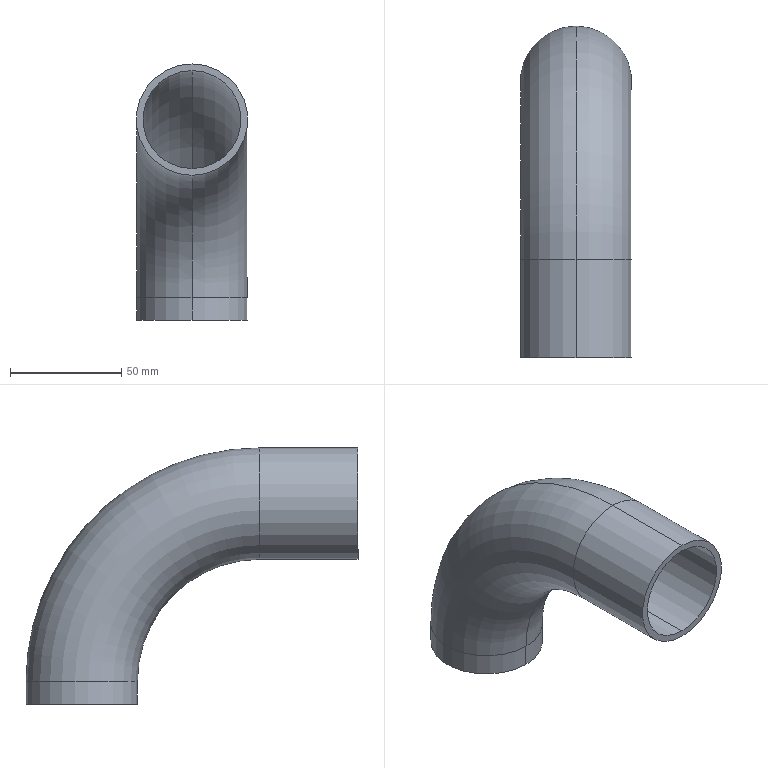Part | SolidWorks | features BaseBody 1 | 1 solid | 14 faces | box 50 x 149 x 115 mm | volume 79585 mm3 | cylinder 8 | torus 4 | plane 2 | commonest cylinder face diameters 44 x4 50 x4
STEP:
#1=CARTESIAN_POINT('',(0.,75.,-80.));
#2=VERTEX_POINT('',#1);
#3=CARTESIAN_POINT('',(0.,125.,-80.));
#4=VERTEX_POINT('',#3);
#5=CARTESIAN_POINT('',(0.,100.,-80.));
#6=DIRECTION('',(0.,0.,1.));
#7=DIRECTION('',(0.,-1.,0.));
#8=AXIS2_PLACEMENT_3D('',#5,#6,#7);
#9=CIRCLE('',#8,25.);
#10=EDGE_CURVE('',#2,#4,#9,.T.);
#11=ORIENTED_EDGE('',*,*,#10,.T.);
#12=CARTESIAN_POINT('',(0.,20.,25.));
#13=VERTEX_POINT('',#12);
#14=CARTESIAN_POINT('',(0.,20.,-80.));
#15=DIRECTION('',(1.,0.,0.));
#16=DIRECTION('',(0.,0.,-1.));
#17=AXIS2_PLACEMENT_3D('',#14,#15,#16);
#18=CIRCLE('',#17,105.);
#19=EDGE_CURVE('',#4,#13,#18,.T.);
#20=ORIENTED_EDGE('',*,*,#19,.T.);
#21=CARTESIAN_POINT('',(0.,20.,-25.));
#22=VERTEX_POINT('',#21);
#23=CARTESIAN_POINT('',(0.,20.,0.));
#24=DIRECTION('',(0.,-1.,0.));
#25=DIRECTION('',(0.,0.,-1.));
#26=AXIS2_PLACEMENT_3D('',#23,#24,#25);
#27=CIRCLE('',#26,25.);
#28=EDGE_CURVE('',#22,#13,#27,.T.);
#29=ORIENTED_EDGE('',*,*,#28,.F.);
#30=CARTESIAN_POINT('',(0.,20.,-80.));
#31=DIRECTION('',(1.,0.,0.));
#32=DIRECTION('',(0.,0.,-1.));
#33=AXIS2_PLACEMENT_3D('',#30,#31,#32);
#34=CIRCLE('',#33,55.);
#35=EDGE_CURVE('',#2,#22,#34,.T.);
#36=ORIENTED_EDGE('',*,*,#35,.F.);
#37=EDGE_LOOP('',(#11,#20,#29,#36));
#38=FACE_OUTER_BOUND('',#37,.T.);
#39=CARTESIAN_POINT('',(0.,20.,-80.));
#40=DIRECTION('',(1.,0.,0.));
#41=DIRECTION('',(0.,0.,1.));
#42=AXIS2_PLACEMENT_3D('',#39,#40,#41);
#43=TOROIDAL_SURFACE('',#42,80.,25.);
#44=ADVANCED_FACE('',(#38),#43,.T.);
#45=CARTESIAN_POINT('',(0.,122.,-80.));
#46=VERTEX_POINT('',#45);
#47=CARTESIAN_POINT('',(0.,78.,-80.));
#48=VERTEX_POINT('',#47);
#49=CARTESIAN_POINT('',(0.,100.,-80.));
#50=DIRECTION('',(0.,0.,1.));
#51=DIRECTION('',(0.,-1.,0.));
#52=AXIS2_PLACEMENT_3D('',#49,#50,#51);
#53=CIRCLE('',#52,22.);
#54=EDGE_CURVE('',#46,#48,#53,.T.);
#55=ORIENTED_EDGE('',*,*,#54,.F.);
#56=CARTESIAN_POINT('',(0.,20.,22.));
#57=VERTEX_POINT('',#56);
#58=CARTESIAN_POINT('',(0.,20.,-80.));
#59=DIRECTION('',(1.,0.,0.));
#60=DIRECTION('',(0.,0.,-1.));
#61=AXIS2_PLACEMENT_3D('',#58,#59,#60);
#62=CIRCLE('',#61,102.);
#63=EDGE_CURVE('',#46,#57,#62,.T.);
#64=ORIENTED_EDGE('',*,*,#63,.T.);
#65=CARTESIAN_POINT('',(0.,20.,-22.));
#66=VERTEX_POINT('',#65);
#67=CARTESIAN_POINT('',(0.,20.,0.));
#68=DIRECTION('',(0.,-1.,0.));
#69=DIRECTION('',(0.,0.,-1.));
#70=AXIS2_PLACEMENT_3D('',#67,#68,#69);
#71=CIRCLE('',#70,22.);
#72=EDGE_CURVE('',#57,#66,#71,.T.);
#73=ORIENTED_EDGE('',*,*,#72,.T.);
#74=CARTESIAN_POINT('',(0.,20.,-80.));
#75=DIRECTION('',(1.,0.,0.));
#76=DIRECTION('',(0.,0.,-1.));
#77=AXIS2_PLACEMENT_3D('',#74,#75,#76);
#78=CIRCLE('',#77,58.);
#79=EDGE_CURVE('',#48,#66,#78,.T.);
#80=ORIENTED_EDGE('',*,*,#79,.F.);
#81=EDGE_LOOP('',(#55,#64,#73,#80));
#82=FACE_OUTER_BOUND('',#81,.T.);
#83=CARTESIAN_POINT('',(0.,20.,-80.));
#84=DIRECTION('',(1.,0.,0.));
#85=DIRECTION('',(0.,0.,1.));
#86=AXIS2_PLACEMENT_3D('',#83,#84,#85);
#87=TOROIDAL_SURFACE('',#86,80.,22.);
#88=ADVANCED_FACE('',(#82),#87,.F.);
#89=CARTESIAN_POINT('',(0.,20.,0.));
#90=DIRECTION('',(0.,-1.,0.));
#91=DIRECTION('',(0.,0.,-1.));
#92=AXIS2_PLACEMENT_3D('',#89,#90,#91);
#93=CIRCLE('',#92,25.);
#94=EDGE_CURVE('',#13,#22,#93,.T.);
#95=ORIENTED_EDGE('',*,*,#94,.T.);
#96=CARTESIAN_POINT('',(0.,-24.,-25.));
#97=VERTEX_POINT('',#96);
#98=CARTESIAN_POINT('',(0.,20.,-25.));
#99=DIRECTION('',(0.,-1.,0.));
#100=VECTOR('',#99,1000.);
#101=LINE('',#98,#100);
#102=EDGE_CURVE('',#22,#97,#101,.T.);
#103=ORIENTED_EDGE('',*,*,#102,.T.);
#104=CARTESIAN_POINT('',(0.,-24.,25.));
#105=VERTEX_POINT('',#104);
#106=CARTESIAN_POINT('',(0.,-24.,0.));
#107=DIRECTION('',(0.,-1.,0.));
#108=DIRECTION('',(0.,0.,-1.));
#109=AXIS2_PLACEMENT_3D('',#106,#107,#108);
#110=CIRCLE('',#109,25.);
#111=EDGE_CURVE('',#105,#97,#110,.T.);
#112=ORIENTED_EDGE('',*,*,#111,.F.);
#113=CARTESIAN_POINT('',(0.,20.,25.));
#114=DIRECTION('',(0.,-1.,0.));
#115=VECTOR('',#114,1000.);
#116=LINE('',#113,#115);
#117=EDGE_CURVE('',#13,#105,#116,.T.);
#118=ORIENTED_EDGE('',*,*,#117,.F.);
#119=EDGE_LOOP('',(#95,#103,#112,#118));
#120=FACE_OUTER_BOUND('',#119,.T.);
#121=CARTESIAN_POINT('',(0.,20.,0.));
#122=DIRECTION('',(0.,-1.,0.));
#123=DIRECTION('',(0.,0.,1.));
#124=AXIS2_PLACEMENT_3D('',#121,#122,#123);
#125=CYLINDRICAL_SURFACE('',#124,25.);
#126=ADVANCED_FACE('',(#120),#125,.T.);
#127=CARTESIAN_POINT('',(0.,20.,0.));
#128=DIRECTION('',(0.,-1.,0.));
#129=DIRECTION('',(0.,0.,-1.));
#130=AXIS2_PLACEMENT_3D('',#127,#128,#129);
#131=CIRCLE('',#130,22.);
#132=EDGE_CURVE('',#66,#57,#131,.T.);
#133=ORIENTED_EDGE('',*,*,#132,.F.);
#134=CARTESIAN_POINT('',(0.,-24.,-22.));
#135=VERTEX_POINT('',#134);
#136=CARTESIAN_POINT('',(0.,20.,-22.));
#137=DIRECTION('',(0.,-1.,0.));
#138=VECTOR('',#137,1000.);
#139=LINE('',#136,#138);
#140=EDGE_CURVE('',#66,#135,#139,.T.);
#141=ORIENTED_EDGE('',*,*,#140,.T.);
#142=CARTESIAN_POINT('',(0.,-24.,22.));
#143=VERTEX_POINT('',#142);
#144=CARTESIAN_POINT('',(0.,-24.,0.));
#145=DIRECTION('',(0.,-1.,0.));
#146=DIRECTION('',(0.,0.,-1.));
#147=AXIS2_PLACEMENT_3D('',#144,#145,#146);
#148=CIRCLE('',#147,22.);
#149=EDGE_CURVE('',#135,#143,#148,.T.);
#150=ORIENTED_EDGE('',*,*,#149,.T.);
#151=CARTESIAN_POINT('',(0.,20.,22.));
#152=DIRECTION('',(0.,-1.,0.));
#153=VECTOR('',#152,1000.);
#154=LINE('',#151,#153);
#155=EDGE_CURVE('',#57,#143,#154,.T.);
#156=ORIENTED_EDGE('',*,*,#155,.F.);
#157=EDGE_LOOP('',(#133,#141,#150,#156));
#158=FACE_OUTER_BOUND('',#157,.T.);
#159=CARTESIAN_POINT('',(0.,20.,0.));
#160=DIRECTION('',(0.,-1.,0.));
#161=DIRECTION('',(0.,0.,1.));
#162=AXIS2_PLACEMENT_3D('',#159,#160,#161);
#163=CYLINDRICAL_SURFACE('',#162,22.);
#164=ADVANCED_FACE('',(#158),#163,.F.);
#165=CARTESIAN_POINT('',(0.,100.,-80.));
#166=DIRECTION('',(0.,0.,1.));
#167=DIRECTION('',(0.,-1.,0.));
#168=AXIS2_PLACEMENT_3D('',#165,#166,#167);
#169=CIRCLE('',#168,22.);
#170=EDGE_CURVE('',#48,#46,#169,.T.);
#171=ORIENTED_EDGE('',*,*,#170,.T.);
#172=CARTESIAN_POINT('',(0.,122.,-90.));
#173=VERTEX_POINT('',#172);
#174=CARTESIAN_POINT('',(0.,122.,-80.));
#175=DIRECTION('',(0.,0.,-1.));
#176=VECTOR('',#175,1000.);
#177=LINE('',#174,#176);
#178=EDGE_CURVE('',#46,#173,#177,.T.);
#179=ORIENTED_EDGE('',*,*,#178,.T.);
#180=CARTESIAN_POINT('',(0.,78.,-90.));
#181=VERTEX_POINT('',#180);
#182=CARTESIAN_POINT('',(0.,100.,-90.));
#183=DIRECTION('',(0.,0.,1.));
#184=DIRECTION('',(0.,-1.,0.));
#185=AXIS2_PLACEMENT_3D('',#182,#183,#184);
#186=CIRCLE('',#185,22.);
#187=EDGE_CURVE('',#181,#173,#186,.T.);
#188=ORIENTED_EDGE('',*,*,#187,.F.);
#189=CARTESIAN_POINT('',(0.,78.,-80.));
#190=DIRECTION('',(0.,0.,-1.));
#191=VECTOR('',#190,1000.);
#192=LINE('',#189,#191);
#193=EDGE_CURVE('',#48,#181,#192,.T.);
#194=ORIENTED_EDGE('',*,*,#193,.F.);
#195=EDGE_LOOP('',(#171,#179,#188,#194));
#196=FACE_OUTER_BOUND('',#195,.T.);
#197=CARTESIAN_POINT('',(0.,100.,-80.));
#198=DIRECTION('',(0.,0.,-1.));
#199=DIRECTION('',(0.,-1.,0.));
#200=AXIS2_PLACEMENT_3D('',#197,#198,#199);
#201=CYLINDRICAL_SURFACE('',#200,22.);
#202=ADVANCED_FACE('',(#196),#201,.F.);
#203=CARTESIAN_POINT('',(0.,100.,-80.));
#204=DIRECTION('',(0.,0.,1.));
#205=DIRECTION('',(0.,-1.,0.));
#206=AXIS2_PLACEMENT_3D('',#203,#204,#205);
#207=CIRCLE('',#206,25.);
#208=EDGE_CURVE('',#4,#2,#207,.T.);
#209=ORIENTED_EDGE('',*,*,#208,.F.);
#210=CARTESIAN_POINT('',(0.,125.,-90.));
#211=VERTEX_POINT('',#210);
#212=CARTESIAN_POINT('',(0.,125.,-80.));
#213=DIRECTION('',(0.,0.,-1.));
#214=VECTOR('',#213,1000.);
#215=LINE('',#212,#214);
#216=EDGE_CURVE('',#4,#211,#215,.T.);
#217=ORIENTED_EDGE('',*,*,#216,.T.);
#218=CARTESIAN_POINT('',(0.,75.,-90.));
#219=VERTEX_POINT('',#218);
#220=CARTESIAN_POINT('',(0.,100.,-90.));
#221=DIRECTION('',(0.,0.,1.));
#222=DIRECTION('',(0.,-1.,0.));
#223=AXIS2_PLACEMENT_3D('',#220,#221,#222);
#224=CIRCLE('',#223,25.);
#225=EDGE_CURVE('',#211,#219,#224,.T.);
#226=ORIENTED_EDGE('',*,*,#225,.T.);
#227=CARTESIAN_POINT('',(0.,75.,-80.));
#228=DIRECTION('',(0.,0.,-1.));
#229=VECTOR('',#228,1000.);
#230=LINE('',#227,#229);
#231=EDGE_CURVE('',#2,#219,#230,.T.);
#232=ORIENTED_EDGE('',*,*,#231,.F.);
#233=EDGE_LOOP('',(#209,#217,#226,#232));
#234=FACE_OUTER_BOUND('',#233,.T.);
#235=CARTESIAN_POINT('',(0.,100.,-80.));
#236=DIRECTION('',(0.,0.,-1.));
#237=DIRECTION('',(0.,-1.,0.));
#238=AXIS2_PLACEMENT_3D('',#235,#236,#237);
#239=CYLINDRICAL_SURFACE('',#238,25.);
#240=ADVANCED_FACE('',(#234),#239,.T.);
#241=CARTESIAN_POINT('',(0.,100.,-90.));
#242=DIRECTION('',(0.,0.,1.));
#243=DIRECTION('',(0.,-1.,0.));
#244=AXIS2_PLACEMENT_3D('',#241,#242,#243);
#245=CIRCLE('',#244,25.);
#246=EDGE_CURVE('',#219,#211,#245,.T.);
#247=ORIENTED_EDGE('',*,*,#246,.F.);
#248=ORIENTED_EDGE('',*,*,#225,.F.);
#249=EDGE_LOOP('',(#247,#248));
#250=FACE_OUTER_BOUND('',#249,.T.);
#251=ORIENTED_EDGE('',*,*,#187,.T.);
#252=CARTESIAN_POINT('',(0.,100.,-90.));
#253=DIRECTION('',(0.,0.,1.));
#254=DIRECTION('',(0.,-1.,0.));
#255=AXIS2_PLACEMENT_3D('',#252,#253,#254);
#256=CIRCLE('',#255,22.);
#257=EDGE_CURVE('',#173,#181,#256,.T.);
#258=ORIENTED_EDGE('',*,*,#257,.T.);
#259=EDGE_LOOP('',(#251,#258));
#260=FACE_BOUND('',#259,.T.);
#261=CARTESIAN_POINT('',(0.,100.,-90.));
#262=DIRECTION('',(0.,0.,1.));
#263=DIRECTION('',(0.,-1.,0.));
#264=AXIS2_PLACEMENT_3D('',#261,#262,#263);
#265=PLANE('',#264);
#266=ADVANCED_FACE('',(#250,#260),#265,.F.);
#267=ORIENTED_EDGE('',*,*,#111,.T.);
#268=CARTESIAN_POINT('',(0.,-24.,0.));
#269=DIRECTION('',(0.,-1.,0.));
#270=DIRECTION('',(0.,0.,-1.));
#271=AXIS2_PLACEMENT_3D('',#268,#269,#270);
#272=CIRCLE('',#271,25.);
#273=EDGE_CURVE('',#97,#105,#272,.T.);
#274=ORIENTED_EDGE('',*,*,#273,.T.);
#275=EDGE_LOOP('',(#267,#274));
#276=FACE_OUTER_BOUND('',#275,.T.);
#277=CARTESIAN_POINT('',(0.,-24.,0.));
#278=DIRECTION('',(0.,-1.,0.));
#279=DIRECTION('',(0.,0.,-1.));
#280=AXIS2_PLACEMENT_3D('',#277,#278,#279);
#281=CIRCLE('',#280,22.);
#282=EDGE_CURVE('',#143,#135,#281,.T.);
#283=ORIENTED_EDGE('',*,*,#282,.F.);
#284=ORIENTED_EDGE('',*,*,#149,.F.);
#285=EDGE_LOOP('',(#283,#284));
#286=FACE_BOUND('',#285,.T.);
#287=CARTESIAN_POINT('',(0.,-24.,0.));
#288=DIRECTION('',(0.,-1.,0.));
#289=DIRECTION('',(-1.,0.,0.));
#290=AXIS2_PLACEMENT_3D('',#287,#288,#289);
#291=PLANE('',#290);
#292=ADVANCED_FACE('',(#276,#286),#291,.T.);
#293=ORIENTED_EDGE('',*,*,#216,.F.);
#294=ORIENTED_EDGE('',*,*,#10,.F.);
#295=ORIENTED_EDGE('',*,*,#231,.T.);
#296=ORIENTED_EDGE('',*,*,#246,.T.);
#297=EDGE_LOOP('',(#293,#294,#295,#296));
#298=FACE_OUTER_BOUND('',#297,.T.);
#299=CARTESIAN_POINT('',(0.,100.,-80.));
#300=DIRECTION('',(0.,0.,-1.));
#301=DIRECTION('',(0.,-1.,0.));
#302=AXIS2_PLACEMENT_3D('',#299,#300,#301);
#303=CYLINDRICAL_SURFACE('',#302,25.);
#304=ADVANCED_FACE('',(#298),#303,.T.);
#305=ORIENTED_EDGE('',*,*,#178,.F.);
#306=ORIENTED_EDGE('',*,*,#54,.T.);
#307=ORIENTED_EDGE('',*,*,#193,.T.);
#308=ORIENTED_EDGE('',*,*,#257,.F.);
#309=EDGE_LOOP('',(#305,#306,#307,#308));
#310=FACE_OUTER_BOUND('',#309,.T.);
#311=CARTESIAN_POINT('',(0.,100.,-80.));
#312=DIRECTION('',(0.,0.,-1.));
#313=DIRECTION('',(0.,-1.,0.));
#314=AXIS2_PLACEMENT_3D('',#311,#312,#313);
#315=CYLINDRICAL_SURFACE('',#314,22.);
#316=ADVANCED_FACE('',(#310),#315,.F.);
#317=ORIENTED_EDGE('',*,*,#63,.F.);
#318=ORIENTED_EDGE('',*,*,#170,.F.);
#319=ORIENTED_EDGE('',*,*,#79,.T.);
#320=ORIENTED_EDGE('',*,*,#132,.T.);
#321=EDGE_LOOP('',(#317,#318,#319,#320));
#322=FACE_OUTER_BOUND('',#321,.T.);
#323=CARTESIAN_POINT('',(0.,20.,-80.));
#324=DIRECTION('',(1.,0.,0.));
#325=DIRECTION('',(0.,0.,1.));
#326=AXIS2_PLACEMENT_3D('',#323,#324,#325);
#327=TOROIDAL_SURFACE('',#326,80.,22.);
#328=ADVANCED_FACE('',(#322),#327,.F.);
#329=ORIENTED_EDGE('',*,*,#19,.F.);
#330=ORIENTED_EDGE('',*,*,#208,.T.);
#331=ORIENTED_EDGE('',*,*,#35,.T.);
#332=ORIENTED_EDGE('',*,*,#94,.F.);
#333=EDGE_LOOP('',(#329,#330,#331,#332));
#334=FACE_OUTER_BOUND('',#333,.T.);
#335=CARTESIAN_POINT('',(0.,20.,-80.));
#336=DIRECTION('',(1.,0.,0.));
#337=DIRECTION('',(0.,0.,1.));
#338=AXIS2_PLACEMENT_3D('',#335,#336,#337);
#339=TOROIDAL_SURFACE('',#338,80.,25.);
#340=ADVANCED_FACE('',(#334),#339,.T.);
#341=ORIENTED_EDGE('',*,*,#140,.F.);
#342=ORIENTED_EDGE('',*,*,#72,.F.);
#343=ORIENTED_EDGE('',*,*,#155,.T.);
#344=ORIENTED_EDGE('',*,*,#282,.T.);
#345=EDGE_LOOP('',(#341,#342,#343,#344));
#346=FACE_OUTER_BOUND('',#345,.T.);
#347=CARTESIAN_POINT('',(0.,20.,0.));
#348=DIRECTION('',(0.,-1.,0.));
#349=DIRECTION('',(0.,0.,1.));
#350=AXIS2_PLACEMENT_3D('',#347,#348,#349);
#351=CYLINDRICAL_SURFACE('',#350,22.);
#352=ADVANCED_FACE('',(#346),#351,.F.);
#353=ORIENTED_EDGE('',*,*,#102,.F.);
#354=ORIENTED_EDGE('',*,*,#28,.T.);
#355=ORIENTED_EDGE('',*,*,#117,.T.);
#356=ORIENTED_EDGE('',*,*,#273,.F.);
#357=EDGE_LOOP('',(#353,#354,#355,#356));
#358=FACE_OUTER_BOUND('',#357,.T.);
#359=CARTESIAN_POINT('',(0.,20.,0.));
#360=DIRECTION('',(0.,-1.,0.));
#361=DIRECTION('',(0.,0.,1.));
#362=AXIS2_PLACEMENT_3D('',#359,#360,#361);
#363=CYLINDRICAL_SURFACE('',#362,25.);
#364=ADVANCED_FACE('',(#358),#363,.T.);
#365=CLOSED_SHELL('',(#44,#88,#126,#164,#202,#240,#266,#292,#304,#316,#328,#340,#352,#364));
#366=MANIFOLD_SOLID_BREP('',#365);
#367=CARTESIAN_POINT('',(0.,0.,0.));
#368=DIRECTION('',(0.,0.,1.));
#369=DIRECTION('',(1.,0.,0.));
#370=AXIS2_PLACEMENT_3D('',#367,#368,#369);
#371=(LENGTH_UNIT()NAMED_UNIT(*)SI_UNIT(.MILLI.,.METRE.));
#372=UNCERTAINTY_MEASURE_WITH_UNIT(LENGTH_MEASURE(0.00001),#371,'','');
#373=(NAMED_UNIT(*)PLANE_ANGLE_UNIT()SI_UNIT($,.RADIAN.));
#374=(NAMED_UNIT(*)SI_UNIT($,.STERADIAN.)SOLID_ANGLE_UNIT());
#375=(GEOMETRIC_REPRESENTATION_CONTEXT(3)GLOBAL_UNCERTAINTY_ASSIGNED_CONTEXT((#372))GLOBAL_UNIT_ASSIGNED_CONTEXT((#371,#373,#374))REPRESENTATION_CONTEXT('',''));
#376=ADVANCED_BREP_SHAPE_REPRESENTATION('',(#366,#370),#375);